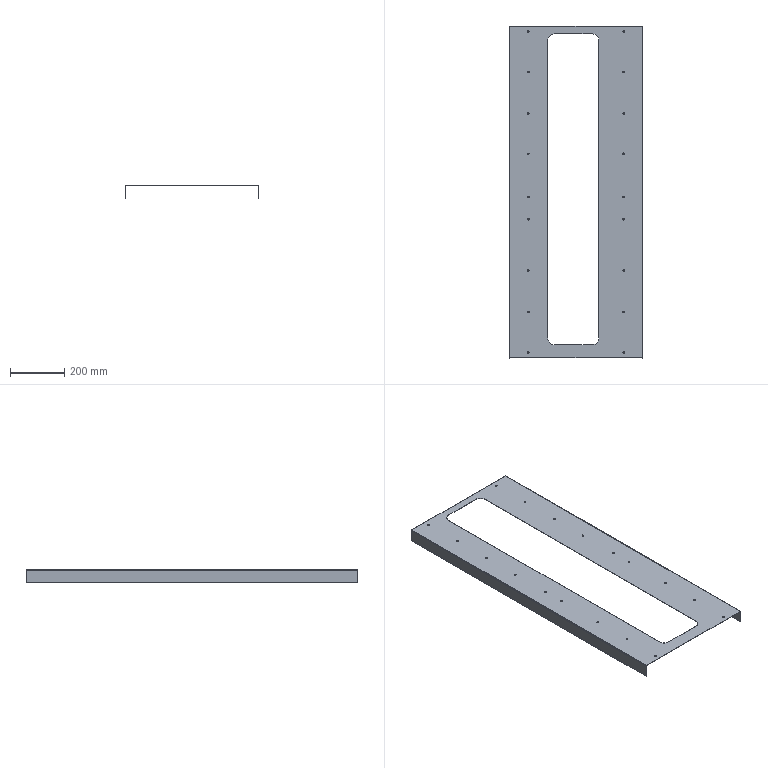Part | SolidWorks | features Cut 3, EdgeFlange 1, FlatPattern 1, SMBaseFlange 1, SheetMetal 1 | 1 solid | 66 faces | box 495 x 1228 x 48 mm | volume 602812 mm3 | cylinder 44 | plane 22 | commonest cylinder face diameters 6.5 x34 50 x4 2.4 x2 4.8 x2 6.393 x2